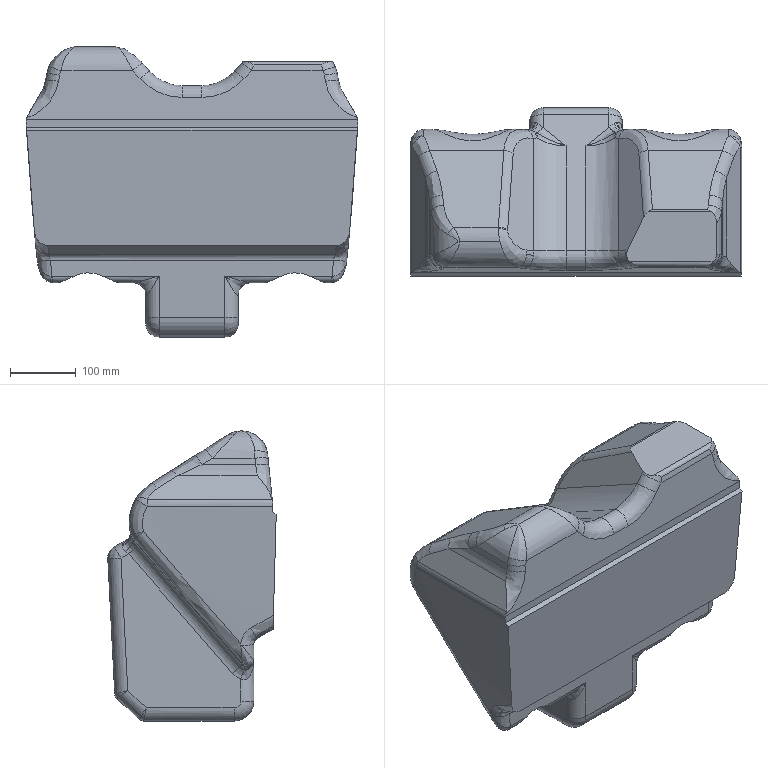Part | SolidWorks | features BaseBody 2 | 2 solids | 339 faces | box 502.867 x 255.374 x 439.801 mm | volume 51406988 mm3 | spline 166 | cylinder 119 | plane 50 | torus 4 | commonest cylinder face diameters 40 x31 34 x29 14 x9 20 x9 74 x7 80 x7